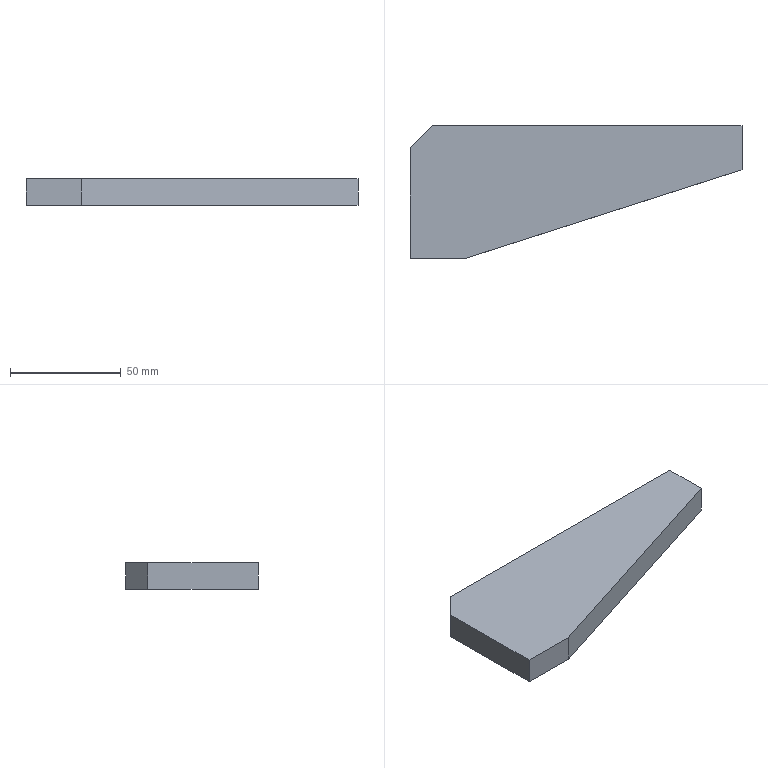Part | STEP file | Rib 7 | 1 solid | 8 faces | box 150 x 60 x 12 mm | volume 77400 mm3 | plane 8
STEP:
#1=CARTESIAN_POINT('',(0.,0.,0.));
#2=DIRECTION('',(0.,0.,1.));
#3=DIRECTION('',(1.,0.,0.));
#4=AXIS2_PLACEMENT_3D('',#1,#2,#3);
#5=CARTESIAN_POINT('',(-1127.,-180.,0.));
#6=VERTEX_POINT('',#5);
#7=CARTESIAN_POINT('',(-1127.,-160.,0.));
#8=VERTEX_POINT('',#7);
#9=CARTESIAN_POINT('',(-1127.,-160.,0.));
#10=DIRECTION('',(0.,1.,0.));
#11=VECTOR('',#10,1.);
#12=LINE('',#9,#11);
#13=CARTESIAN_POINT('',(-1127.,-160.,12.));
#14=DIRECTION('',(-1.,0.,0.));
#15=DIRECTION('',(0.,0.,1.));
#16=AXIS2_PLACEMENT_3D('',#13,#14,#15);
#17=PLANE('',#16);
#18=CARTESIAN_POINT('',(-12.,0.));
#19=DIRECTION('',(0.,1.));
#20=VECTOR('',#19,1.);
#21=LINE('',#18,#20);
#22=(GEOMETRIC_REPRESENTATION_CONTEXT(2)PARAMETRIC_REPRESENTATION_CONTEXT()REPRESENTATION_CONTEXT('',''));
#23=DEFINITIONAL_REPRESENTATION('',(#21),#22);
#24=PCURVE('',#17,#23);
#25=CARTESIAN_POINT('',(-1127.,-220.,0.));
#26=DIRECTION('',(0.,0.,-1.));
#27=DIRECTION('',(-1.,0.,0.));
#28=AXIS2_PLACEMENT_3D('',#25,#26,#27);
#29=PLANE('',#28);
#30=CARTESIAN_POINT('',(0.,60.));
#31=DIRECTION('',(0.,1.));
#32=VECTOR('',#31,1.);
#33=LINE('',#30,#32);
#34=(GEOMETRIC_REPRESENTATION_CONTEXT(2)PARAMETRIC_REPRESENTATION_CONTEXT()REPRESENTATION_CONTEXT('',''));
#35=DEFINITIONAL_REPRESENTATION('',(#33),#34);
#36=PCURVE('',#29,#35);
#37=SURFACE_CURVE('',#12,(#24,#36),.PCURVE_S1.);
#38=EDGE_CURVE('',#6,#8,#37,.T.);
#39=ORIENTED_EDGE('',*,*,#38,.T.);
#40=CARTESIAN_POINT('',(-1127.,-160.,12.));
#41=VERTEX_POINT('',#40);
#42=CARTESIAN_POINT('',(-1127.,-160.,12.));
#43=DIRECTION('',(0.,0.,-1.));
#44=VECTOR('',#43,1.);
#45=LINE('',#42,#44);
#46=CARTESIAN_POINT('',(0.,0.));
#47=DIRECTION('',(-1.,0.));
#48=VECTOR('',#47,1.);
#49=LINE('',#46,#48);
#50=(GEOMETRIC_REPRESENTATION_CONTEXT(2)PARAMETRIC_REPRESENTATION_CONTEXT()REPRESENTATION_CONTEXT('',''));
#51=DEFINITIONAL_REPRESENTATION('',(#49),#50);
#52=PCURVE('',#17,#51);
#53=CARTESIAN_POINT('',(-1267.,-160.,12.));
#54=DIRECTION('',(0.,-1.,0.));
#55=DIRECTION('',(0.,0.,-1.));
#56=AXIS2_PLACEMENT_3D('',#53,#54,#55);
#57=PLANE('',#56);
#58=CARTESIAN_POINT('',(0.,140.));
#59=DIRECTION('',(1.,0.));
#60=VECTOR('',#59,1.);
#61=LINE('',#58,#60);
#62=(GEOMETRIC_REPRESENTATION_CONTEXT(2)PARAMETRIC_REPRESENTATION_CONTEXT()REPRESENTATION_CONTEXT('',''));
#63=DEFINITIONAL_REPRESENTATION('',(#61),#62);
#64=PCURVE('',#57,#63);
#65=SURFACE_CURVE('',#45,(#52,#64),.PCURVE_S1.);
#66=EDGE_CURVE('',#41,#8,#65,.T.);
#67=ORIENTED_EDGE('',*,*,#66,.F.);
#68=CARTESIAN_POINT('',(-1127.,-180.,12.));
#69=VERTEX_POINT('',#68);
#70=CARTESIAN_POINT('',(-1127.,-160.,12.));
#71=DIRECTION('',(0.,1.,0.));
#72=VECTOR('',#71,1.);
#73=LINE('',#70,#72);
#74=CARTESIAN_POINT('',(0.,0.));
#75=DIRECTION('',(0.,1.));
#76=VECTOR('',#75,1.);
#77=LINE('',#74,#76);
#78=(GEOMETRIC_REPRESENTATION_CONTEXT(2)PARAMETRIC_REPRESENTATION_CONTEXT()REPRESENTATION_CONTEXT('',''));
#79=DEFINITIONAL_REPRESENTATION('',(#77),#78);
#80=PCURVE('',#17,#79);
#81=CARTESIAN_POINT('',(-1127.,-220.,12.));
#82=DIRECTION('',(0.,0.,-1.));
#83=DIRECTION('',(-1.,0.,0.));
#84=AXIS2_PLACEMENT_3D('',#81,#82,#83);
#85=PLANE('',#84);
#86=CARTESIAN_POINT('',(0.,60.));
#87=DIRECTION('',(0.,1.));
#88=VECTOR('',#87,1.);
#89=LINE('',#86,#88);
#90=(GEOMETRIC_REPRESENTATION_CONTEXT(2)PARAMETRIC_REPRESENTATION_CONTEXT()REPRESENTATION_CONTEXT('',''));
#91=DEFINITIONAL_REPRESENTATION('',(#89),#90);
#92=PCURVE('',#85,#91);
#93=SURFACE_CURVE('',#73,(#80,#92),.PCURVE_S1.);
#94=EDGE_CURVE('',#69,#41,#93,.T.);
#95=ORIENTED_EDGE('',*,*,#94,.F.);
#96=CARTESIAN_POINT('',(-1127.,-180.,12.));
#97=DIRECTION('',(0.,0.,-1.));
#98=VECTOR('',#97,1.);
#99=LINE('',#96,#98);
#100=CARTESIAN_POINT('',(0.,-20.));
#101=DIRECTION('',(-1.,0.));
#102=VECTOR('',#101,1.);
#103=LINE('',#100,#102);
#104=(GEOMETRIC_REPRESENTATION_CONTEXT(2)PARAMETRIC_REPRESENTATION_CONTEXT()REPRESENTATION_CONTEXT('',''));
#105=DEFINITIONAL_REPRESENTATION('',(#103),#104);
#106=PCURVE('',#17,#105);
#107=CARTESIAN_POINT('',(-1127.,-180.,12.));
#108=DIRECTION('',(-0.3048,0.9524,0.));
#109=DIRECTION('',(-0.9524,-0.3048,0.));
#110=AXIS2_PLACEMENT_3D('',#107,#108,#109);
#111=PLANE('',#110);
#112=CARTESIAN_POINT('',(0.,0.));
#113=DIRECTION('',(0.,-1.));
#114=VECTOR('',#113,1.);
#115=LINE('',#112,#114);
#116=(GEOMETRIC_REPRESENTATION_CONTEXT(2)PARAMETRIC_REPRESENTATION_CONTEXT()REPRESENTATION_CONTEXT('',''));
#117=DEFINITIONAL_REPRESENTATION('',(#115),#116);
#118=PCURVE('',#111,#117);
#119=SURFACE_CURVE('',#99,(#106,#118),.PCURVE_S1.);
#120=EDGE_CURVE('',#69,#6,#119,.T.);
#121=ORIENTED_EDGE('',*,*,#120,.T.);
#122=EDGE_LOOP('',(#39,#67,#95,#121));
#123=FACE_BOUND('',#122,.T.);
#124=ADVANCED_FACE('',(#123),#17,.F.);
#125=CARTESIAN_POINT('',(-1267.,-160.,0.));
#126=VERTEX_POINT('',#125);
#127=CARTESIAN_POINT('',(-1267.,-160.,0.));
#128=DIRECTION('',(-1.,0.,0.));
#129=VECTOR('',#128,1.);
#130=LINE('',#127,#129);
#131=CARTESIAN_POINT('',(12.,0.));
#132=DIRECTION('',(0.,-1.));
#133=VECTOR('',#132,1.);
#134=LINE('',#131,#133);
#135=(GEOMETRIC_REPRESENTATION_CONTEXT(2)PARAMETRIC_REPRESENTATION_CONTEXT()REPRESENTATION_CONTEXT('',''));
#136=DEFINITIONAL_REPRESENTATION('',(#134),#135);
#137=PCURVE('',#57,#136);
#138=CARTESIAN_POINT('',(140.,60.));
#139=DIRECTION('',(1.,0.));
#140=VECTOR('',#139,1.);
#141=LINE('',#138,#140);
#142=(GEOMETRIC_REPRESENTATION_CONTEXT(2)PARAMETRIC_REPRESENTATION_CONTEXT()REPRESENTATION_CONTEXT('',''));
#143=DEFINITIONAL_REPRESENTATION('',(#141),#142);
#144=PCURVE('',#29,#143);
#145=SURFACE_CURVE('',#130,(#137,#144),.PCURVE_S1.);
#146=EDGE_CURVE('',#8,#126,#145,.T.);
#147=ORIENTED_EDGE('',*,*,#146,.T.);
#148=CARTESIAN_POINT('',(-1267.,-160.,12.));
#149=VERTEX_POINT('',#148);
#150=CARTESIAN_POINT('',(-1267.,-160.,12.));
#151=DIRECTION('',(0.,0.,-1.));
#152=VECTOR('',#151,1.);
#153=LINE('',#150,#152);
#154=CARTESIAN_POINT('',(0.,0.));
#155=DIRECTION('',(1.,0.));
#156=VECTOR('',#155,1.);
#157=LINE('',#154,#156);
#158=(GEOMETRIC_REPRESENTATION_CONTEXT(2)PARAMETRIC_REPRESENTATION_CONTEXT()REPRESENTATION_CONTEXT('',''));
#159=DEFINITIONAL_REPRESENTATION('',(#157),#158);
#160=PCURVE('',#57,#159);
#161=CARTESIAN_POINT('',(-1277.,-170.,12.));
#162=DIRECTION('',(0.7071,-0.7071,0.));
#163=DIRECTION('',(0.7071,0.7071,0.));
#164=AXIS2_PLACEMENT_3D('',#161,#162,#163);
#165=PLANE('',#164);
#166=CARTESIAN_POINT('',(14.142,0.));
#167=DIRECTION('',(0.,-1.));
#168=VECTOR('',#167,1.);
#169=LINE('',#166,#168);
#170=(GEOMETRIC_REPRESENTATION_CONTEXT(2)PARAMETRIC_REPRESENTATION_CONTEXT()REPRESENTATION_CONTEXT('',''));
#171=DEFINITIONAL_REPRESENTATION('',(#169),#170);
#172=PCURVE('',#165,#171);
#173=SURFACE_CURVE('',#153,(#160,#172),.PCURVE_S1.);
#174=EDGE_CURVE('',#149,#126,#173,.T.);
#175=ORIENTED_EDGE('',*,*,#174,.F.);
#176=CARTESIAN_POINT('',(-1267.,-160.,12.));
#177=DIRECTION('',(-1.,0.,0.));
#178=VECTOR('',#177,1.);
#179=LINE('',#176,#178);
#180=CARTESIAN_POINT('',(0.,0.));
#181=DIRECTION('',(0.,-1.));
#182=VECTOR('',#181,1.);
#183=LINE('',#180,#182);
#184=(GEOMETRIC_REPRESENTATION_CONTEXT(2)PARAMETRIC_REPRESENTATION_CONTEXT()REPRESENTATION_CONTEXT('',''));
#185=DEFINITIONAL_REPRESENTATION('',(#183),#184);
#186=PCURVE('',#57,#185);
#187=CARTESIAN_POINT('',(140.,60.));
#188=DIRECTION('',(1.,0.));
#189=VECTOR('',#188,1.);
#190=LINE('',#187,#189);
#191=(GEOMETRIC_REPRESENTATION_CONTEXT(2)PARAMETRIC_REPRESENTATION_CONTEXT()REPRESENTATION_CONTEXT('',''));
#192=DEFINITIONAL_REPRESENTATION('',(#190),#191);
#193=PCURVE('',#85,#192);
#194=SURFACE_CURVE('',#179,(#186,#193),.PCURVE_S1.);
#195=EDGE_CURVE('',#41,#149,#194,.T.);
#196=ORIENTED_EDGE('',*,*,#195,.F.);
#197=ORIENTED_EDGE('',*,*,#66,.T.);
#198=EDGE_LOOP('',(#147,#175,#196,#197));
#199=FACE_BOUND('',#198,.T.);
#200=ADVANCED_FACE('',(#199),#57,.F.);
#201=CARTESIAN_POINT('',(-1277.,-170.,0.));
#202=VERTEX_POINT('',#201);
#203=CARTESIAN_POINT('',(-1277.,-170.,0.));
#204=DIRECTION('',(-0.7071,-0.7071,0.));
#205=VECTOR('',#204,1.);
#206=LINE('',#203,#205);
#207=CARTESIAN_POINT('',(0.,-12.));
#208=DIRECTION('',(-1.,0.));
#209=VECTOR('',#208,1.);
#210=LINE('',#207,#209);
#211=(GEOMETRIC_REPRESENTATION_CONTEXT(2)PARAMETRIC_REPRESENTATION_CONTEXT()REPRESENTATION_CONTEXT('',''));
#212=DEFINITIONAL_REPRESENTATION('',(#210),#211);
#213=PCURVE('',#165,#212);
#214=CARTESIAN_POINT('',(150.,50.));
#215=DIRECTION('',(0.7071,-0.7071));
#216=VECTOR('',#215,1.);
#217=LINE('',#214,#216);
#218=(GEOMETRIC_REPRESENTATION_CONTEXT(2)PARAMETRIC_REPRESENTATION_CONTEXT()REPRESENTATION_CONTEXT('',''));
#219=DEFINITIONAL_REPRESENTATION('',(#217),#218);
#220=PCURVE('',#29,#219);
#221=SURFACE_CURVE('',#206,(#213,#220),.PCURVE_S1.);
#222=EDGE_CURVE('',#126,#202,#221,.T.);
#223=ORIENTED_EDGE('',*,*,#222,.T.);
#224=CARTESIAN_POINT('',(-1277.,-170.,12.));
#225=VERTEX_POINT('',#224);
#226=CARTESIAN_POINT('',(-1277.,-170.,12.));
#227=DIRECTION('',(0.,0.,-1.));
#228=VECTOR('',#227,1.);
#229=LINE('',#226,#228);
#230=CARTESIAN_POINT('',(0.,0.));
#231=DIRECTION('',(0.,-1.));
#232=VECTOR('',#231,1.);
#233=LINE('',#230,#232);
#234=(GEOMETRIC_REPRESENTATION_CONTEXT(2)PARAMETRIC_REPRESENTATION_CONTEXT()REPRESENTATION_CONTEXT('',''));
#235=DEFINITIONAL_REPRESENTATION('',(#233),#234);
#236=PCURVE('',#165,#235);
#237=CARTESIAN_POINT('',(-1277.,-220.,12.));
#238=DIRECTION('',(1.,0.,0.));
#239=DIRECTION('',(0.,0.,-1.));
#240=AXIS2_PLACEMENT_3D('',#237,#238,#239);
#241=PLANE('',#240);
#242=CARTESIAN_POINT('',(0.,50.));
#243=DIRECTION('',(1.,0.));
#244=VECTOR('',#243,1.);
#245=LINE('',#242,#244);
#246=(GEOMETRIC_REPRESENTATION_CONTEXT(2)PARAMETRIC_REPRESENTATION_CONTEXT()REPRESENTATION_CONTEXT('',''));
#247=DEFINITIONAL_REPRESENTATION('',(#245),#246);
#248=PCURVE('',#241,#247);
#249=SURFACE_CURVE('',#229,(#236,#248),.PCURVE_S1.);
#250=EDGE_CURVE('',#225,#202,#249,.T.);
#251=ORIENTED_EDGE('',*,*,#250,.F.);
#252=CARTESIAN_POINT('',(-1277.,-170.,12.));
#253=DIRECTION('',(-0.7071,-0.7071,0.));
#254=VECTOR('',#253,1.);
#255=LINE('',#252,#254);
#256=CARTESIAN_POINT('',(0.,0.));
#257=DIRECTION('',(-1.,0.));
#258=VECTOR('',#257,1.);
#259=LINE('',#256,#258);
#260=(GEOMETRIC_REPRESENTATION_CONTEXT(2)PARAMETRIC_REPRESENTATION_CONTEXT()REPRESENTATION_CONTEXT('',''));
#261=DEFINITIONAL_REPRESENTATION('',(#259),#260);
#262=PCURVE('',#165,#261);
#263=CARTESIAN_POINT('',(150.,50.));
#264=DIRECTION('',(0.7071,-0.7071));
#265=VECTOR('',#264,1.);
#266=LINE('',#263,#265);
#267=(GEOMETRIC_REPRESENTATION_CONTEXT(2)PARAMETRIC_REPRESENTATION_CONTEXT()REPRESENTATION_CONTEXT('',''));
#268=DEFINITIONAL_REPRESENTATION('',(#266),#267);
#269=PCURVE('',#85,#268);
#270=SURFACE_CURVE('',#255,(#262,#269),.PCURVE_S1.);
#271=EDGE_CURVE('',#149,#225,#270,.T.);
#272=ORIENTED_EDGE('',*,*,#271,.F.);
#273=ORIENTED_EDGE('',*,*,#174,.T.);
#274=EDGE_LOOP('',(#223,#251,#272,#273));
#275=FACE_BOUND('',#274,.T.);
#276=ADVANCED_FACE('',(#275),#165,.F.);
#277=CARTESIAN_POINT('',(-1277.,-220.,0.));
#278=VERTEX_POINT('',#277);
#279=CARTESIAN_POINT('',(-1277.,-220.,0.));
#280=DIRECTION('',(0.,-1.,0.));
#281=VECTOR('',#280,1.);
#282=LINE('',#279,#281);
#283=CARTESIAN_POINT('',(12.,0.));
#284=DIRECTION('',(0.,-1.));
#285=VECTOR('',#284,1.);
#286=LINE('',#283,#285);
#287=(GEOMETRIC_REPRESENTATION_CONTEXT(2)PARAMETRIC_REPRESENTATION_CONTEXT()REPRESENTATION_CONTEXT('',''));
#288=DEFINITIONAL_REPRESENTATION('',(#286),#287);
#289=PCURVE('',#241,#288);
#290=CARTESIAN_POINT('',(150.,0.));
#291=DIRECTION('',(0.,-1.));
#292=VECTOR('',#291,1.);
#293=LINE('',#290,#292);
#294=(GEOMETRIC_REPRESENTATION_CONTEXT(2)PARAMETRIC_REPRESENTATION_CONTEXT()REPRESENTATION_CONTEXT('',''));
#295=DEFINITIONAL_REPRESENTATION('',(#293),#294);
#296=PCURVE('',#29,#295);
#297=SURFACE_CURVE('',#282,(#289,#296),.PCURVE_S1.);
#298=EDGE_CURVE('',#202,#278,#297,.T.);
#299=ORIENTED_EDGE('',*,*,#298,.T.);
#300=CARTESIAN_POINT('',(-1277.,-220.,12.));
#301=VERTEX_POINT('',#300);
#302=CARTESIAN_POINT('',(-1277.,-220.,12.));
#303=DIRECTION('',(0.,0.,-1.));
#304=VECTOR('',#303,1.);
#305=LINE('',#302,#304);
#306=CARTESIAN_POINT('',(0.,0.));
#307=DIRECTION('',(1.,0.));
#308=VECTOR('',#307,1.);
#309=LINE('',#306,#308);
#310=(GEOMETRIC_REPRESENTATION_CONTEXT(2)PARAMETRIC_REPRESENTATION_CONTEXT()REPRESENTATION_CONTEXT('',''));
#311=DEFINITIONAL_REPRESENTATION('',(#309),#310);
#312=PCURVE('',#241,#311);
#313=CARTESIAN_POINT('',(-1252.,-220.,12.));
#314=DIRECTION('',(0.,1.,0.));
#315=DIRECTION('',(-1.,0.,0.));
#316=AXIS2_PLACEMENT_3D('',#313,#314,#315);
#317=PLANE('',#316);
#318=CARTESIAN_POINT('',(25.,0.));
#319=DIRECTION('',(0.,-1.));
#320=VECTOR('',#319,1.);
#321=LINE('',#318,#320);
#322=(GEOMETRIC_REPRESENTATION_CONTEXT(2)PARAMETRIC_REPRESENTATION_CONTEXT()REPRESENTATION_CONTEXT('',''));
#323=DEFINITIONAL_REPRESENTATION('',(#321),#322);
#324=PCURVE('',#317,#323);
#325=SURFACE_CURVE('',#305,(#312,#324),.PCURVE_S1.);
#326=EDGE_CURVE('',#301,#278,#325,.T.);
#327=ORIENTED_EDGE('',*,*,#326,.F.);
#328=CARTESIAN_POINT('',(-1277.,-220.,12.));
#329=DIRECTION('',(0.,-1.,0.));
#330=VECTOR('',#329,1.);
#331=LINE('',#328,#330);
#332=CARTESIAN_POINT('',(0.,0.));
#333=DIRECTION('',(0.,-1.));
#334=VECTOR('',#333,1.);
#335=LINE('',#332,#334);
#336=(GEOMETRIC_REPRESENTATION_CONTEXT(2)PARAMETRIC_REPRESENTATION_CONTEXT()REPRESENTATION_CONTEXT('',''));
#337=DEFINITIONAL_REPRESENTATION('',(#335),#336);
#338=PCURVE('',#241,#337);
#339=CARTESIAN_POINT('',(150.,0.));
#340=DIRECTION('',(0.,-1.));
#341=VECTOR('',#340,1.);
#342=LINE('',#339,#341);
#343=(GEOMETRIC_REPRESENTATION_CONTEXT(2)PARAMETRIC_REPRESENTATION_CONTEXT()REPRESENTATION_CONTEXT('',''));
#344=DEFINITIONAL_REPRESENTATION('',(#342),#343);
#345=PCURVE('',#85,#344);
#346=SURFACE_CURVE('',#331,(#338,#345),.PCURVE_S1.);
#347=EDGE_CURVE('',#225,#301,#346,.T.);
#348=ORIENTED_EDGE('',*,*,#347,.F.);
#349=ORIENTED_EDGE('',*,*,#250,.T.);
#350=EDGE_LOOP('',(#299,#327,#348,#349));
#351=FACE_BOUND('',#350,.T.);
#352=ADVANCED_FACE('',(#351),#241,.F.);
#353=CARTESIAN_POINT('',(-1252.,-220.,0.));
#354=VERTEX_POINT('',#353);
#355=CARTESIAN_POINT('',(-1252.,-220.,0.));
#356=DIRECTION('',(1.,0.,0.));
#357=VECTOR('',#356,1.);
#358=LINE('',#355,#357);
#359=CARTESIAN_POINT('',(0.,-12.));
#360=DIRECTION('',(-1.,0.));
#361=VECTOR('',#360,1.);
#362=LINE('',#359,#361);
#363=(GEOMETRIC_REPRESENTATION_CONTEXT(2)PARAMETRIC_REPRESENTATION_CONTEXT()REPRESENTATION_CONTEXT('',''));
#364=DEFINITIONAL_REPRESENTATION('',(#362),#363);
#365=PCURVE('',#317,#364);
#366=CARTESIAN_POINT('',(125.,0.));
#367=DIRECTION('',(-1.,0.));
#368=VECTOR('',#367,1.);
#369=LINE('',#366,#368);
#370=(GEOMETRIC_REPRESENTATION_CONTEXT(2)PARAMETRIC_REPRESENTATION_CONTEXT()REPRESENTATION_CONTEXT('',''));
#371=DEFINITIONAL_REPRESENTATION('',(#369),#370);
#372=PCURVE('',#29,#371);
#373=SURFACE_CURVE('',#358,(#365,#372),.PCURVE_S1.);
#374=EDGE_CURVE('',#278,#354,#373,.T.);
#375=ORIENTED_EDGE('',*,*,#374,.T.);
#376=CARTESIAN_POINT('',(-1252.,-220.,12.));
#377=VERTEX_POINT('',#376);
#378=CARTESIAN_POINT('',(-1252.,-220.,12.));
#379=DIRECTION('',(0.,0.,-1.));
#380=VECTOR('',#379,1.);
#381=LINE('',#378,#380);
#382=CARTESIAN_POINT('',(0.,0.));
#383=DIRECTION('',(0.,-1.));
#384=VECTOR('',#383,1.);
#385=LINE('',#382,#384);
#386=(GEOMETRIC_REPRESENTATION_CONTEXT(2)PARAMETRIC_REPRESENTATION_CONTEXT()REPRESENTATION_CONTEXT('',''));
#387=DEFINITIONAL_REPRESENTATION('',(#385),#386);
#388=PCURVE('',#317,#387);
#389=CARTESIAN_POINT('',(131.244,0.));
#390=DIRECTION('',(0.,-1.));
#391=VECTOR('',#390,1.);
#392=LINE('',#389,#391);
#393=(GEOMETRIC_REPRESENTATION_CONTEXT(2)PARAMETRIC_REPRESENTATION_CONTEXT()REPRESENTATION_CONTEXT('',''));
#394=DEFINITIONAL_REPRESENTATION('',(#392),#393);
#395=PCURVE('',#111,#394);
#396=SURFACE_CURVE('',#381,(#388,#395),.PCURVE_S1.);
#397=EDGE_CURVE('',#377,#354,#396,.T.);
#398=ORIENTED_EDGE('',*,*,#397,.F.);
#399=CARTESIAN_POINT('',(-1252.,-220.,12.));
#400=DIRECTION('',(1.,0.,0.));
#401=VECTOR('',#400,1.);
#402=LINE('',#399,#401);
#403=CARTESIAN_POINT('',(0.,0.));
#404=DIRECTION('',(-1.,0.));
#405=VECTOR('',#404,1.);
#406=LINE('',#403,#405);
#407=(GEOMETRIC_REPRESENTATION_CONTEXT(2)PARAMETRIC_REPRESENTATION_CONTEXT()REPRESENTATION_CONTEXT('',''));
#408=DEFINITIONAL_REPRESENTATION('',(#406),#407);
#409=PCURVE('',#317,#408);
#410=CARTESIAN_POINT('',(125.,0.));
#411=DIRECTION('',(-1.,0.));
#412=VECTOR('',#411,1.);
#413=LINE('',#410,#412);
#414=(GEOMETRIC_REPRESENTATION_CONTEXT(2)PARAMETRIC_REPRESENTATION_CONTEXT()REPRESENTATION_CONTEXT('',''));
#415=DEFINITIONAL_REPRESENTATION('',(#413),#414);
#416=PCURVE('',#85,#415);
#417=SURFACE_CURVE('',#402,(#409,#416),.PCURVE_S1.);
#418=EDGE_CURVE('',#301,#377,#417,.T.);
#419=ORIENTED_EDGE('',*,*,#418,.F.);
#420=ORIENTED_EDGE('',*,*,#326,.T.);
#421=EDGE_LOOP('',(#375,#398,#419,#420));
#422=FACE_BOUND('',#421,.T.);
#423=ADVANCED_FACE('',(#422),#317,.F.);
#424=CARTESIAN_POINT('',(-1127.,-180.,0.));
#425=DIRECTION('',(0.9524,0.3048,0.));
#426=VECTOR('',#425,1.);
#427=LINE('',#424,#426);
#428=CARTESIAN_POINT('',(0.,-12.));
#429=DIRECTION('',(-1.,0.));
#430=VECTOR('',#429,1.);
#431=LINE('',#428,#430);
#432=(GEOMETRIC_REPRESENTATION_CONTEXT(2)PARAMETRIC_REPRESENTATION_CONTEXT()REPRESENTATION_CONTEXT('',''));
#433=DEFINITIONAL_REPRESENTATION('',(#431),#432);
#434=PCURVE('',#111,#433);
#435=CARTESIAN_POINT('',(0.,40.));
#436=DIRECTION('',(-0.9524,0.3048));
#437=VECTOR('',#436,1.);
#438=LINE('',#435,#437);
#439=(GEOMETRIC_REPRESENTATION_CONTEXT(2)PARAMETRIC_REPRESENTATION_CONTEXT()REPRESENTATION_CONTEXT('',''));
#440=DEFINITIONAL_REPRESENTATION('',(#438),#439);
#441=PCURVE('',#29,#440);
#442=SURFACE_CURVE('',#427,(#434,#441),.PCURVE_S1.);
#443=EDGE_CURVE('',#354,#6,#442,.T.);
#444=ORIENTED_EDGE('',*,*,#443,.T.);
#445=ORIENTED_EDGE('',*,*,#120,.F.);
#446=CARTESIAN_POINT('',(-1127.,-180.,12.));
#447=DIRECTION('',(0.9524,0.3048,0.));
#448=VECTOR('',#447,1.);
#449=LINE('',#446,#448);
#450=CARTESIAN_POINT('',(0.,0.));
#451=DIRECTION('',(-1.,0.));
#452=VECTOR('',#451,1.);
#453=LINE('',#450,#452);
#454=(GEOMETRIC_REPRESENTATION_CONTEXT(2)PARAMETRIC_REPRESENTATION_CONTEXT()REPRESENTATION_CONTEXT('',''));
#455=DEFINITIONAL_REPRESENTATION('',(#453),#454);
#456=PCURVE('',#111,#455);
#457=CARTESIAN_POINT('',(0.,40.));
#458=DIRECTION('',(-0.9524,0.3048));
#459=VECTOR('',#458,1.);
#460=LINE('',#457,#459);
#461=(GEOMETRIC_REPRESENTATION_CONTEXT(2)PARAMETRIC_REPRESENTATION_CONTEXT()REPRESENTATION_CONTEXT('',''));
#462=DEFINITIONAL_REPRESENTATION('',(#460),#461);
#463=PCURVE('',#85,#462);
#464=SURFACE_CURVE('',#449,(#456,#463),.PCURVE_S1.);
#465=EDGE_CURVE('',#377,#69,#464,.T.);
#466=ORIENTED_EDGE('',*,*,#465,.F.);
#467=ORIENTED_EDGE('',*,*,#397,.T.);
#468=EDGE_LOOP('',(#444,#445,#466,#467));
#469=FACE_BOUND('',#468,.T.);
#470=ADVANCED_FACE('',(#469),#111,.F.);
#471=ORIENTED_EDGE('',*,*,#94,.T.);
#472=ORIENTED_EDGE('',*,*,#195,.T.);
#473=ORIENTED_EDGE('',*,*,#271,.T.);
#474=ORIENTED_EDGE('',*,*,#347,.T.);
#475=ORIENTED_EDGE('',*,*,#418,.T.);
#476=ORIENTED_EDGE('',*,*,#465,.T.);
#477=EDGE_LOOP('',(#471,#472,#473,#474,#475,#476));
#478=FACE_BOUND('',#477,.T.);
#479=ADVANCED_FACE('',(#478),#85,.F.);
#480=ORIENTED_EDGE('',*,*,#38,.F.);
#481=ORIENTED_EDGE('',*,*,#443,.F.);
#482=ORIENTED_EDGE('',*,*,#374,.F.);
#483=ORIENTED_EDGE('',*,*,#298,.F.);
#484=ORIENTED_EDGE('',*,*,#222,.F.);
#485=ORIENTED_EDGE('',*,*,#146,.F.);
#486=EDGE_LOOP('',(#480,#481,#482,#483,#484,#485));
#487=FACE_BOUND('',#486,.T.);
#488=ADVANCED_FACE('',(#487),#29,.T.);
#489=CLOSED_SHELL('',(#124,#200,#276,#352,#423,#470,#479,#488));
#490=MANIFOLD_SOLID_BREP('',#489);
#491=(LENGTH_UNIT()NAMED_UNIT(*)SI_UNIT(.MILLI.,.METRE.));
#492=UNCERTAINTY_MEASURE_WITH_UNIT(LENGTH_MEASURE(0.0000001),#491,'','');
#493=(NAMED_UNIT(*)PLANE_ANGLE_UNIT()SI_UNIT($,.RADIAN.));
#494=(NAMED_UNIT(*)SI_UNIT($,.STERADIAN.)SOLID_ANGLE_UNIT());
#495=(GEOMETRIC_REPRESENTATION_CONTEXT(3)GLOBAL_UNCERTAINTY_ASSIGNED_CONTEXT((#492))GLOBAL_UNIT_ASSIGNED_CONTEXT((#491,#493,#494))REPRESENTATION_CONTEXT('',''));
#496=ADVANCED_BREP_SHAPE_REPRESENTATION('',(#4,#490),#495);